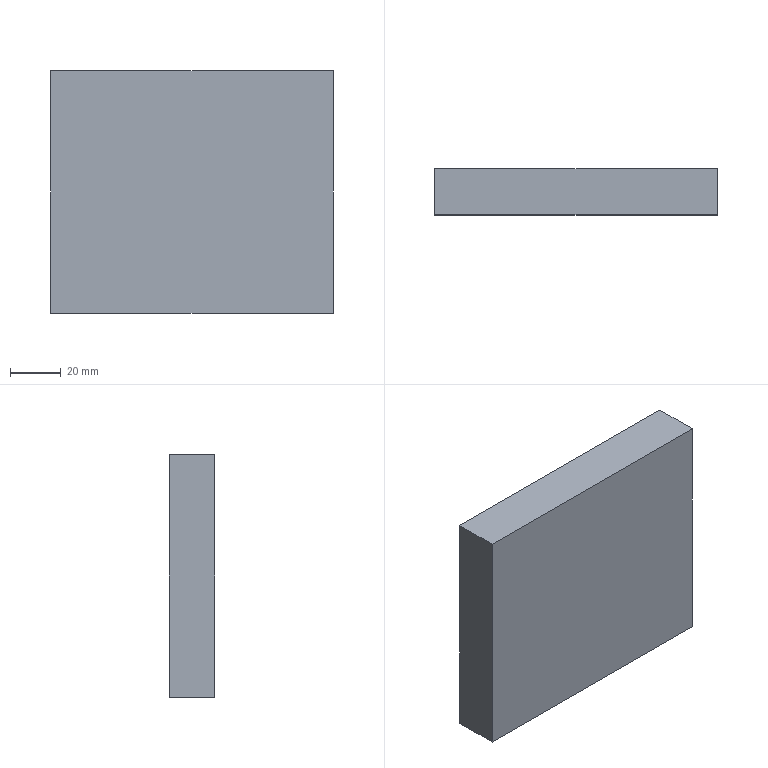Part | STEP file | ASND-0110-Part 13g1kk | 1 solid | 6 faces | box 111 x 18 x 95 mm | volume 189810 mm3 | plane 6
STEP:
#1=CARTESIAN_POINT('',(0.,0.,0.));
#2=DIRECTION('',(0.,0.,1.));
#3=DIRECTION('',(1.,0.,0.));
#4=AXIS2_PLACEMENT_3D('',#1,#2,#3);
#5=CARTESIAN_POINT('',(-53.,18.,-5.));
#6=VERTEX_POINT('',#5);
#7=CARTESIAN_POINT('',(58.,18.,-5.));
#8=VERTEX_POINT('',#7);
#9=CARTESIAN_POINT('',(-73.,18.,-5.));
#10=DIRECTION('',(1.,0.,0.));
#11=VECTOR('',#10,1.);
#12=LINE('',#9,#11);
#13=CARTESIAN_POINT('',(-58.,20.,-5.));
#14=DIRECTION('',(0.,0.,-1.));
#15=DIRECTION('',(0.7071,0.7071,0.));
#16=AXIS2_PLACEMENT_3D('',#13,#14,#15);
#17=PLANE('',#16);
#18=CARTESIAN_POINT('',(-12.021,-9.192));
#19=DIRECTION('',(0.7071,0.7071));
#20=VECTOR('',#19,1.);
#21=LINE('',#18,#20);
#22=(GEOMETRIC_REPRESENTATION_CONTEXT(2)PARAMETRIC_REPRESENTATION_CONTEXT()REPRESENTATION_CONTEXT('',''));
#23=DEFINITIONAL_REPRESENTATION('',(#21),#22);
#24=PCURVE('',#17,#23);
#25=CARTESIAN_POINT('',(0.,18.,0.));
#26=DIRECTION('',(0.,1.,0.));
#27=DIRECTION('',(0.7071,0.,0.7071));
#28=AXIS2_PLACEMENT_3D('',#25,#26,#27);
#29=PLANE('',#28);
#30=CARTESIAN_POINT('',(-55.154,-48.083));
#31=DIRECTION('',(0.7071,0.7071));
#32=VECTOR('',#31,1.);
#33=LINE('',#30,#32);
#34=(GEOMETRIC_REPRESENTATION_CONTEXT(2)PARAMETRIC_REPRESENTATION_CONTEXT()REPRESENTATION_CONTEXT('',''));
#35=DEFINITIONAL_REPRESENTATION('',(#33),#34);
#36=PCURVE('',#29,#35);
#37=SURFACE_CURVE('',#12,(#24,#36),.PCURVE_S1.);
#38=EDGE_CURVE('',#6,#8,#37,.T.);
#39=ORIENTED_EDGE('',*,*,#38,.F.);
#40=CARTESIAN_POINT('',(-53.,0.,-5.));
#41=VERTEX_POINT('',#40);
#42=CARTESIAN_POINT('',(-53.,0.,-5.));
#43=DIRECTION('',(0.,1.,0.));
#44=VECTOR('',#43,1.);
#45=LINE('',#42,#44);
#46=CARTESIAN_POINT('',(-10.607,17.678));
#47=DIRECTION('',(0.7071,-0.7071));
#48=VECTOR('',#47,1.);
#49=LINE('',#46,#48);
#50=(GEOMETRIC_REPRESENTATION_CONTEXT(2)PARAMETRIC_REPRESENTATION_CONTEXT()REPRESENTATION_CONTEXT('',''));
#51=DEFINITIONAL_REPRESENTATION('',(#49),#50);
#52=PCURVE('',#17,#51);
#53=CARTESIAN_POINT('',(-53.,177.785,36.));
#54=DIRECTION('',(-1.,0.,0.));
#55=DIRECTION('',(0.,0.7071,0.7071));
#56=AXIS2_PLACEMENT_3D('',#53,#54,#55);
#57=PLANE('',#56);
#58=CARTESIAN_POINT('',(-154.704,-96.721));
#59=DIRECTION('',(0.7071,0.7071));
#60=VECTOR('',#59,1.);
#61=LINE('',#58,#60);
#62=(GEOMETRIC_REPRESENTATION_CONTEXT(2)PARAMETRIC_REPRESENTATION_CONTEXT()REPRESENTATION_CONTEXT('',''));
#63=DEFINITIONAL_REPRESENTATION('',(#61),#62);
#64=PCURVE('',#57,#63);
#65=SURFACE_CURVE('',#45,(#52,#64),.PCURVE_S1.);
#66=EDGE_CURVE('',#41,#6,#65,.T.);
#67=ORIENTED_EDGE('',*,*,#66,.F.);
#68=CARTESIAN_POINT('',(58.,0.,-5.));
#69=VERTEX_POINT('',#68);
#70=CARTESIAN_POINT('',(-73.,0.,-5.));
#71=DIRECTION('',(1.,0.,0.));
#72=VECTOR('',#71,1.);
#73=LINE('',#70,#72);
#74=CARTESIAN_POINT('',(-24.749,3.536));
#75=DIRECTION('',(0.7071,0.7071));
#76=VECTOR('',#75,1.);
#77=LINE('',#74,#76);
#78=(GEOMETRIC_REPRESENTATION_CONTEXT(2)PARAMETRIC_REPRESENTATION_CONTEXT()REPRESENTATION_CONTEXT('',''));
#79=DEFINITIONAL_REPRESENTATION('',(#77),#78);
#80=PCURVE('',#17,#79);
#81=CARTESIAN_POINT('',(0.,0.,0.));
#82=DIRECTION('',(0.,1.,0.));
#83=DIRECTION('',(0.7071,0.,0.7071));
#84=AXIS2_PLACEMENT_3D('',#81,#82,#83);
#85=PLANE('',#84);
#86=CARTESIAN_POINT('',(-55.154,-48.083));
#87=DIRECTION('',(0.7071,0.7071));
#88=VECTOR('',#87,1.);
#89=LINE('',#86,#88);
#90=(GEOMETRIC_REPRESENTATION_CONTEXT(2)PARAMETRIC_REPRESENTATION_CONTEXT()REPRESENTATION_CONTEXT('',''));
#91=DEFINITIONAL_REPRESENTATION('',(#89),#90);
#92=PCURVE('',#85,#91);
#93=SURFACE_CURVE('',#73,(#80,#92),.PCURVE_S1.);
#94=EDGE_CURVE('',#41,#69,#93,.T.);
#95=ORIENTED_EDGE('',*,*,#94,.T.);
#96=CARTESIAN_POINT('',(58.,20.,-5.));
#97=DIRECTION('',(0.,-1.,0.));
#98=VECTOR('',#97,1.);
#99=LINE('',#96,#98);
#100=CARTESIAN_POINT('',(82.024,82.024));
#101=DIRECTION('',(-0.7071,0.7071));
#102=VECTOR('',#101,1.);
#103=LINE('',#100,#102);
#104=(GEOMETRIC_REPRESENTATION_CONTEXT(2)PARAMETRIC_REPRESENTATION_CONTEXT()REPRESENTATION_CONTEXT('',''));
#105=DEFINITIONAL_REPRESENTATION('',(#103),#104);
#106=PCURVE('',#17,#105);
#107=CARTESIAN_POINT('',(58.,20.,-100.));
#108=DIRECTION('',(-1.,0.,0.));
#109=DIRECTION('',(0.,0.7071,0.7071));
#110=AXIS2_PLACEMENT_3D('',#107,#108,#109);
#111=PLANE('',#110);
#112=CARTESIAN_POINT('',(67.175,-67.175));
#113=DIRECTION('',(-0.7071,-0.7071));
#114=VECTOR('',#113,1.);
#115=LINE('',#112,#114);
#116=(GEOMETRIC_REPRESENTATION_CONTEXT(2)PARAMETRIC_REPRESENTATION_CONTEXT()REPRESENTATION_CONTEXT('',''));
#117=DEFINITIONAL_REPRESENTATION('',(#115),#116);
#118=PCURVE('',#111,#117);
#119=SURFACE_CURVE('',#99,(#106,#118),.PCURVE_S1.);
#120=EDGE_CURVE('',#8,#69,#119,.T.);
#121=ORIENTED_EDGE('',*,*,#120,.F.);
#122=EDGE_LOOP('',(#39,#67,#95,#121));
#123=FACE_BOUND('',#122,.T.);
#124=ADVANCED_FACE('',(#123),#17,.F.);
#125=CARTESIAN_POINT('',(58.,18.,-100.));
#126=VERTEX_POINT('',#125);
#127=CARTESIAN_POINT('',(58.,18.,20.));
#128=DIRECTION('',(0.,0.,-1.));
#129=VECTOR('',#128,1.);
#130=LINE('',#127,#129);
#131=CARTESIAN_POINT('',(83.439,-86.267));
#132=DIRECTION('',(-0.7071,0.7071));
#133=VECTOR('',#132,1.);
#134=LINE('',#131,#133);
#135=(GEOMETRIC_REPRESENTATION_CONTEXT(2)PARAMETRIC_REPRESENTATION_CONTEXT()REPRESENTATION_CONTEXT('',''));
#136=DEFINITIONAL_REPRESENTATION('',(#134),#135);
#137=PCURVE('',#111,#136);
#138=CARTESIAN_POINT('',(55.154,26.87));
#139=DIRECTION('',(-0.7071,0.7071));
#140=VECTOR('',#139,1.);
#141=LINE('',#138,#140);
#142=(GEOMETRIC_REPRESENTATION_CONTEXT(2)PARAMETRIC_REPRESENTATION_CONTEXT()REPRESENTATION_CONTEXT('',''));
#143=DEFINITIONAL_REPRESENTATION('',(#141),#142);
#144=PCURVE('',#29,#143);
#145=SURFACE_CURVE('',#130,(#137,#144),.PCURVE_S1.);
#146=EDGE_CURVE('',#8,#126,#145,.T.);
#147=ORIENTED_EDGE('',*,*,#146,.F.);
#148=ORIENTED_EDGE('',*,*,#120,.T.);
#149=CARTESIAN_POINT('',(58.,0.,-100.));
#150=VERTEX_POINT('',#149);
#151=CARTESIAN_POINT('',(58.,0.,20.));
#152=DIRECTION('',(0.,0.,-1.));
#153=VECTOR('',#152,1.);
#154=LINE('',#151,#153);
#155=CARTESIAN_POINT('',(70.711,-98.995));
#156=DIRECTION('',(-0.7071,0.7071));
#157=VECTOR('',#156,1.);
#158=LINE('',#155,#157);
#159=(GEOMETRIC_REPRESENTATION_CONTEXT(2)PARAMETRIC_REPRESENTATION_CONTEXT()REPRESENTATION_CONTEXT('',''));
#160=DEFINITIONAL_REPRESENTATION('',(#158),#159);
#161=PCURVE('',#111,#160);
#162=CARTESIAN_POINT('',(55.154,26.87));
#163=DIRECTION('',(-0.7071,0.7071));
#164=VECTOR('',#163,1.);
#165=LINE('',#162,#164);
#166=(GEOMETRIC_REPRESENTATION_CONTEXT(2)PARAMETRIC_REPRESENTATION_CONTEXT()REPRESENTATION_CONTEXT('',''));
#167=DEFINITIONAL_REPRESENTATION('',(#165),#166);
#168=PCURVE('',#85,#167);
#169=SURFACE_CURVE('',#154,(#161,#168),.PCURVE_S1.);
#170=EDGE_CURVE('',#69,#150,#169,.T.);
#171=ORIENTED_EDGE('',*,*,#170,.T.);
#172=CARTESIAN_POINT('',(58.,20.,-100.));
#173=DIRECTION('',(0.,-1.,0.));
#174=VECTOR('',#173,1.);
#175=LINE('',#172,#174);
#176=CARTESIAN_POINT('',(0.,0.));
#177=DIRECTION('',(-0.7071,-0.7071));
#178=VECTOR('',#177,1.);
#179=LINE('',#176,#178);
#180=(GEOMETRIC_REPRESENTATION_CONTEXT(2)PARAMETRIC_REPRESENTATION_CONTEXT()REPRESENTATION_CONTEXT('',''));
#181=DEFINITIONAL_REPRESENTATION('',(#179),#180);
#182=PCURVE('',#111,#181);
#183=CARTESIAN_POINT('',(-58.,20.,-100.));
#184=DIRECTION('',(0.,0.,1.));
#185=DIRECTION('',(0.7071,0.7071,0.));
#186=AXIS2_PLACEMENT_3D('',#183,#184,#185);
#187=PLANE('',#186);
#188=CARTESIAN_POINT('',(82.024,-82.024));
#189=DIRECTION('',(-0.7071,-0.7071));
#190=VECTOR('',#189,1.);
#191=LINE('',#188,#190);
#192=(GEOMETRIC_REPRESENTATION_CONTEXT(2)PARAMETRIC_REPRESENTATION_CONTEXT()REPRESENTATION_CONTEXT('',''));
#193=DEFINITIONAL_REPRESENTATION('',(#191),#192);
#194=PCURVE('',#187,#193);
#195=SURFACE_CURVE('',#175,(#182,#194),.PCURVE_S1.);
#196=EDGE_CURVE('',#126,#150,#195,.T.);
#197=ORIENTED_EDGE('',*,*,#196,.F.);
#198=EDGE_LOOP('',(#147,#148,#171,#197));
#199=FACE_BOUND('',#198,.T.);
#200=ADVANCED_FACE('',(#199),#111,.F.);
#201=CARTESIAN_POINT('',(-53.,18.,-100.));
#202=VERTEX_POINT('',#201);
#203=CARTESIAN_POINT('',(58.,18.,-100.));
#204=DIRECTION('',(-1.,0.,0.));
#205=VECTOR('',#204,1.);
#206=LINE('',#203,#205);
#207=CARTESIAN_POINT('',(80.61,-83.439));
#208=DIRECTION('',(-0.7071,0.7071));
#209=VECTOR('',#208,1.);
#210=LINE('',#207,#209);
#211=(GEOMETRIC_REPRESENTATION_CONTEXT(2)PARAMETRIC_REPRESENTATION_CONTEXT()REPRESENTATION_CONTEXT('',''));
#212=DEFINITIONAL_REPRESENTATION('',(#210),#211);
#213=PCURVE('',#187,#212);
#214=CARTESIAN_POINT('',(-29.698,111.723));
#215=DIRECTION('',(-0.7071,-0.7071));
#216=VECTOR('',#215,1.);
#217=LINE('',#214,#216);
#218=(GEOMETRIC_REPRESENTATION_CONTEXT(2)PARAMETRIC_REPRESENTATION_CONTEXT()REPRESENTATION_CONTEXT('',''));
#219=DEFINITIONAL_REPRESENTATION('',(#217),#218);
#220=PCURVE('',#29,#219);
#221=SURFACE_CURVE('',#206,(#213,#220),.PCURVE_S1.);
#222=EDGE_CURVE('',#126,#202,#221,.T.);
#223=ORIENTED_EDGE('',*,*,#222,.F.);
#224=ORIENTED_EDGE('',*,*,#196,.T.);
#225=CARTESIAN_POINT('',(-53.,0.,-100.));
#226=VERTEX_POINT('',#225);
#227=CARTESIAN_POINT('',(58.,0.,-100.));
#228=DIRECTION('',(-1.,0.,0.));
#229=VECTOR('',#228,1.);
#230=LINE('',#227,#229);
#231=CARTESIAN_POINT('',(67.882,-96.167));
#232=DIRECTION('',(-0.7071,0.7071));
#233=VECTOR('',#232,1.);
#234=LINE('',#231,#233);
#235=(GEOMETRIC_REPRESENTATION_CONTEXT(2)PARAMETRIC_REPRESENTATION_CONTEXT()REPRESENTATION_CONTEXT('',''));
#236=DEFINITIONAL_REPRESENTATION('',(#234),#235);
#237=PCURVE('',#187,#236);
#238=CARTESIAN_POINT('',(-29.698,111.723));
#239=DIRECTION('',(-0.7071,-0.7071));
#240=VECTOR('',#239,1.);
#241=LINE('',#238,#240);
#242=(GEOMETRIC_REPRESENTATION_CONTEXT(2)PARAMETRIC_REPRESENTATION_CONTEXT()REPRESENTATION_CONTEXT('',''));
#243=DEFINITIONAL_REPRESENTATION('',(#241),#242);
#244=PCURVE('',#85,#243);
#245=SURFACE_CURVE('',#230,(#237,#244),.PCURVE_S1.);
#246=EDGE_CURVE('',#150,#226,#245,.T.);
#247=ORIENTED_EDGE('',*,*,#246,.T.);
#248=CARTESIAN_POINT('',(-53.,20.,-100.));
#249=DIRECTION('',(0.,-1.,0.));
#250=VECTOR('',#249,1.);
#251=LINE('',#248,#250);
#252=CARTESIAN_POINT('',(3.536,-3.536));
#253=DIRECTION('',(-0.7071,-0.7071));
#254=VECTOR('',#253,1.);
#255=LINE('',#252,#254);
#256=(GEOMETRIC_REPRESENTATION_CONTEXT(2)PARAMETRIC_REPRESENTATION_CONTEXT()REPRESENTATION_CONTEXT('',''));
#257=DEFINITIONAL_REPRESENTATION('',(#255),#256);
#258=PCURVE('',#187,#257);
#259=CARTESIAN_POINT('',(-207.737,-15.404));
#260=DIRECTION('',(-0.7071,-0.7071));
#261=VECTOR('',#260,1.);
#262=LINE('',#259,#261);
#263=(GEOMETRIC_REPRESENTATION_CONTEXT(2)PARAMETRIC_REPRESENTATION_CONTEXT()REPRESENTATION_CONTEXT('',''));
#264=DEFINITIONAL_REPRESENTATION('',(#262),#263);
#265=PCURVE('',#57,#264);
#266=SURFACE_CURVE('',#251,(#258,#265),.PCURVE_S1.);
#267=EDGE_CURVE('',#202,#226,#266,.T.);
#268=ORIENTED_EDGE('',*,*,#267,.F.);
#269=EDGE_LOOP('',(#223,#224,#247,#268));
#270=FACE_BOUND('',#269,.T.);
#271=ADVANCED_FACE('',(#270),#187,.F.);
#272=CARTESIAN_POINT('',(-53.,18.,20.));
#273=DIRECTION('',(0.,0.,-1.));
#274=VECTOR('',#273,1.);
#275=LINE('',#272,#274);
#276=CARTESIAN_POINT('',(-23.335,-51.619));
#277=DIRECTION('',(-0.7071,0.7071));
#278=VECTOR('',#277,1.);
#279=LINE('',#276,#278);
#280=(GEOMETRIC_REPRESENTATION_CONTEXT(2)PARAMETRIC_REPRESENTATION_CONTEXT()REPRESENTATION_CONTEXT('',''));
#281=DEFINITIONAL_REPRESENTATION('',(#279),#280);
#282=PCURVE('',#29,#281);
#283=CARTESIAN_POINT('',(-124.299,-101.671));
#284=DIRECTION('',(-0.7071,0.7071));
#285=VECTOR('',#284,1.);
#286=LINE('',#283,#285);
#287=(GEOMETRIC_REPRESENTATION_CONTEXT(2)PARAMETRIC_REPRESENTATION_CONTEXT()REPRESENTATION_CONTEXT('',''));
#288=DEFINITIONAL_REPRESENTATION('',(#286),#287);
#289=PCURVE('',#57,#288);
#290=SURFACE_CURVE('',#275,(#282,#289),.PCURVE_S1.);
#291=EDGE_CURVE('',#6,#202,#290,.T.);
#292=ORIENTED_EDGE('',*,*,#291,.F.);
#293=ORIENTED_EDGE('',*,*,#38,.T.);
#294=ORIENTED_EDGE('',*,*,#146,.T.);
#295=ORIENTED_EDGE('',*,*,#222,.T.);
#296=EDGE_LOOP('',(#292,#293,#294,#295));
#297=FACE_BOUND('',#296,.T.);
#298=ADVANCED_FACE('',(#297),#29,.T.);
#299=ORIENTED_EDGE('',*,*,#94,.F.);
#300=CARTESIAN_POINT('',(-53.,0.,-100.));
#301=DIRECTION('',(0.,0.,1.));
#302=VECTOR('',#301,1.);
#303=LINE('',#300,#302);
#304=CARTESIAN_POINT('',(-108.187,33.234));
#305=DIRECTION('',(0.7071,-0.7071));
#306=VECTOR('',#305,1.);
#307=LINE('',#304,#306);
#308=(GEOMETRIC_REPRESENTATION_CONTEXT(2)PARAMETRIC_REPRESENTATION_CONTEXT()REPRESENTATION_CONTEXT('',''));
#309=DEFINITIONAL_REPRESENTATION('',(#307),#308);
#310=PCURVE('',#85,#309);
#311=CARTESIAN_POINT('',(-221.879,-29.546));
#312=DIRECTION('',(0.7071,-0.7071));
#313=VECTOR('',#312,1.);
#314=LINE('',#311,#313);
#315=(GEOMETRIC_REPRESENTATION_CONTEXT(2)PARAMETRIC_REPRESENTATION_CONTEXT()REPRESENTATION_CONTEXT('',''));
#316=DEFINITIONAL_REPRESENTATION('',(#314),#315);
#317=PCURVE('',#57,#316);
#318=SURFACE_CURVE('',#303,(#310,#317),.PCURVE_S1.);
#319=EDGE_CURVE('',#226,#41,#318,.T.);
#320=ORIENTED_EDGE('',*,*,#319,.F.);
#321=ORIENTED_EDGE('',*,*,#246,.F.);
#322=ORIENTED_EDGE('',*,*,#170,.F.);
#323=EDGE_LOOP('',(#299,#320,#321,#322));
#324=FACE_BOUND('',#323,.T.);
#325=ADVANCED_FACE('',(#324),#85,.F.);
#326=ORIENTED_EDGE('',*,*,#66,.T.);
#327=ORIENTED_EDGE('',*,*,#291,.T.);
#328=ORIENTED_EDGE('',*,*,#267,.T.);
#329=ORIENTED_EDGE('',*,*,#319,.T.);
#330=EDGE_LOOP('',(#326,#327,#328,#329));
#331=FACE_BOUND('',#330,.T.);
#332=ADVANCED_FACE('',(#331),#57,.T.);
#333=CLOSED_SHELL('',(#124,#200,#271,#298,#325,#332));
#334=MANIFOLD_SOLID_BREP('',#333);
#335=(LENGTH_UNIT()NAMED_UNIT(*)SI_UNIT(.MILLI.,.METRE.));
#336=UNCERTAINTY_MEASURE_WITH_UNIT(LENGTH_MEASURE(0.0000001),#335,'','');
#337=(NAMED_UNIT(*)PLANE_ANGLE_UNIT()SI_UNIT($,.RADIAN.));
#338=(NAMED_UNIT(*)SI_UNIT($,.STERADIAN.)SOLID_ANGLE_UNIT());
#339=(GEOMETRIC_REPRESENTATION_CONTEXT(3)GLOBAL_UNCERTAINTY_ASSIGNED_CONTEXT((#336))GLOBAL_UNIT_ASSIGNED_CONTEXT((#335,#337,#338))REPRESENTATION_CONTEXT('',''));
#340=ADVANCED_BREP_SHAPE_REPRESENTATION('',(#4,#334),#339);